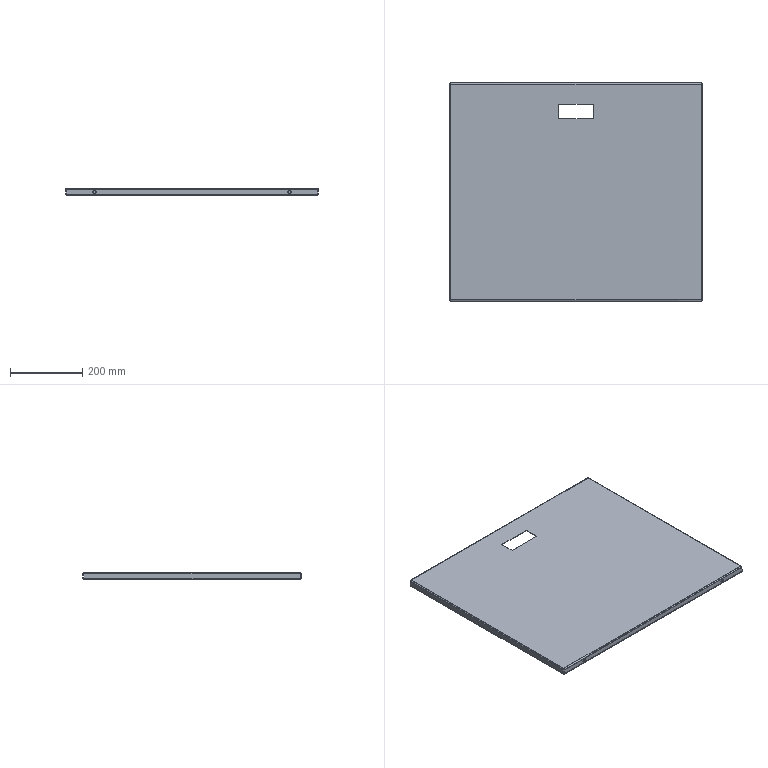Part | SolidWorks | features EdgeFlange 2, FlatPattern 1, HoleWzd 1, SMBaseFlange 1, SheetMetal 1 | 1 solid | 78 faces | box 700 x 605 x 20 mm | volume 761861 mm3 | plane 42 | cylinder 20 | spline 16 | commonest cylinder face diameters 4 x8 7 x8 9 x4